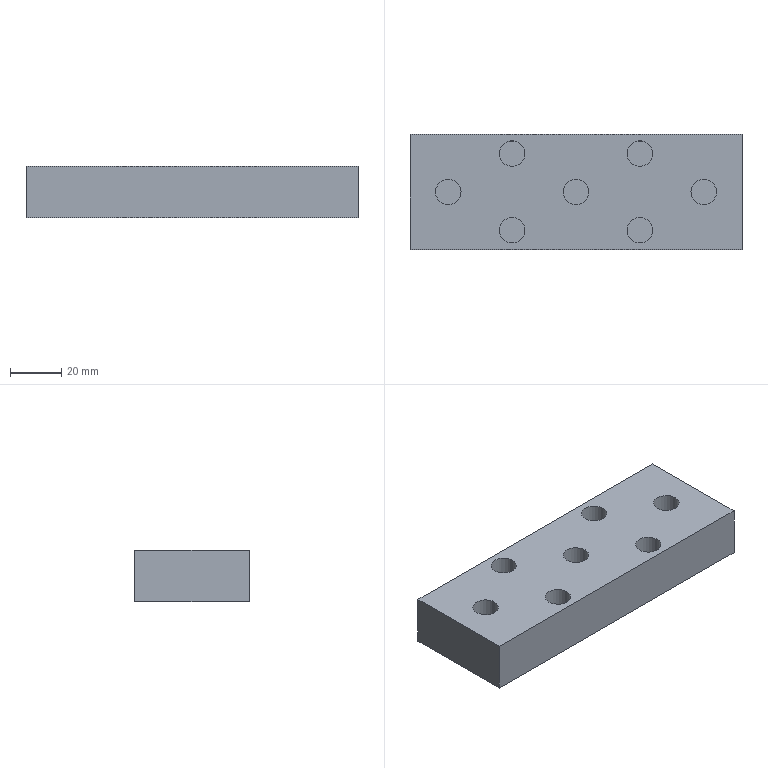Part | NX | 1 solid | 20 faces | box 130 x 45 x 20 mm | volume 111502 mm3 | plane 13 | cylinder 7 | commonest cylinder face diameters 10 x7
STEP:
#1=CARTESIAN_POINT('',(95.,37.5,20.));
#2=VERTEX_POINT('',#1);
#3=CARTESIAN_POINT('',(90.,37.5,20.));
#4=DIRECTION('',(0.,0.,-1.));
#5=DIRECTION('',(1.,0.,0.));
#6=AXIS2_PLACEMENT_3D('',#3,#4,#5);
#7=CIRCLE('',#6,5.);
#8=EDGE_CURVE('',#2,#2,#7,.T.);
#9=ORIENTED_EDGE('',*,*,#8,.T.);
#10=EDGE_LOOP('',(#9));
#11=FACE_BOUND('',#10,.T.);
#12=CARTESIAN_POINT('',(45.,37.5,20.));
#13=VERTEX_POINT('',#12);
#14=CARTESIAN_POINT('',(40.,37.5,20.));
#15=DIRECTION('',(0.,0.,-1.));
#16=DIRECTION('',(1.,0.,0.));
#17=AXIS2_PLACEMENT_3D('',#14,#15,#16);
#18=CIRCLE('',#17,5.);
#19=EDGE_CURVE('',#13,#13,#18,.T.);
#20=ORIENTED_EDGE('',*,*,#19,.T.);
#21=EDGE_LOOP('',(#20));
#22=FACE_BOUND('',#21,.T.);
#23=CARTESIAN_POINT('',(95.,7.5,20.));
#24=VERTEX_POINT('',#23);
#25=CARTESIAN_POINT('',(90.,7.5,20.));
#26=DIRECTION('',(0.,0.,-1.));
#27=DIRECTION('',(1.,0.,0.));
#28=AXIS2_PLACEMENT_3D('',#25,#26,#27);
#29=CIRCLE('',#28,5.);
#30=EDGE_CURVE('',#24,#24,#29,.T.);
#31=ORIENTED_EDGE('',*,*,#30,.T.);
#32=EDGE_LOOP('',(#31));
#33=FACE_BOUND('',#32,.T.);
#34=CARTESIAN_POINT('',(45.,7.5,20.));
#35=VERTEX_POINT('',#34);
#36=CARTESIAN_POINT('',(40.,7.5,20.));
#37=DIRECTION('',(0.,0.,-1.));
#38=DIRECTION('',(1.,0.,0.));
#39=AXIS2_PLACEMENT_3D('',#36,#37,#38);
#40=CIRCLE('',#39,5.);
#41=EDGE_CURVE('',#35,#35,#40,.T.);
#42=ORIENTED_EDGE('',*,*,#41,.T.);
#43=EDGE_LOOP('',(#42));
#44=FACE_BOUND('',#43,.T.);
#45=CARTESIAN_POINT('',(120.,22.5,20.));
#46=VERTEX_POINT('',#45);
#47=CARTESIAN_POINT('',(115.,22.5,20.));
#48=DIRECTION('',(0.,0.,-1.));
#49=DIRECTION('',(1.,0.,0.));
#50=AXIS2_PLACEMENT_3D('',#47,#48,#49);
#51=CIRCLE('',#50,5.);
#52=EDGE_CURVE('',#46,#46,#51,.T.);
#53=ORIENTED_EDGE('',*,*,#52,.T.);
#54=EDGE_LOOP('',(#53));
#55=FACE_BOUND('',#54,.T.);
#56=CARTESIAN_POINT('',(20.,22.5,20.));
#57=VERTEX_POINT('',#56);
#58=CARTESIAN_POINT('',(15.,22.5,20.));
#59=DIRECTION('',(0.,0.,-1.));
#60=DIRECTION('',(1.,0.,0.));
#61=AXIS2_PLACEMENT_3D('',#58,#59,#60);
#62=CIRCLE('',#61,5.);
#63=EDGE_CURVE('',#57,#57,#62,.T.);
#64=ORIENTED_EDGE('',*,*,#63,.T.);
#65=EDGE_LOOP('',(#64));
#66=FACE_BOUND('',#65,.T.);
#67=CARTESIAN_POINT('',(70.,22.5,20.));
#68=VERTEX_POINT('',#67);
#69=CARTESIAN_POINT('',(65.,22.5,20.));
#70=DIRECTION('',(0.,0.,-1.));
#71=DIRECTION('',(1.,0.,0.));
#72=AXIS2_PLACEMENT_3D('',#69,#70,#71);
#73=CIRCLE('',#72,5.);
#74=EDGE_CURVE('',#68,#68,#73,.T.);
#75=ORIENTED_EDGE('',*,*,#74,.T.);
#76=EDGE_LOOP('',(#75));
#77=FACE_BOUND('',#76,.T.);
#78=CARTESIAN_POINT('',(130.,0.,20.));
#79=VERTEX_POINT('',#78);
#80=CARTESIAN_POINT('',(0.,0.,20.));
#81=VERTEX_POINT('',#80);
#82=CARTESIAN_POINT('',(65.,0.,20.));
#83=DIRECTION('',(-1.,0.,0.));
#84=VECTOR('',#83,1000.);
#85=LINE('',#82,#84);
#86=EDGE_CURVE('',#79,#81,#85,.T.);
#87=ORIENTED_EDGE('',*,*,#86,.F.);
#88=CARTESIAN_POINT('',(130.,45.,20.));
#89=VERTEX_POINT('',#88);
#90=CARTESIAN_POINT('',(130.,22.5,20.));
#91=DIRECTION('',(0.,-1.,0.));
#92=VECTOR('',#91,1000.);
#93=LINE('',#90,#92);
#94=EDGE_CURVE('',#89,#79,#93,.T.);
#95=ORIENTED_EDGE('',*,*,#94,.F.);
#96=CARTESIAN_POINT('',(0.,45.,20.));
#97=VERTEX_POINT('',#96);
#98=CARTESIAN_POINT('',(65.,45.,20.));
#99=DIRECTION('',(1.,0.,0.));
#100=VECTOR('',#99,1000.);
#101=LINE('',#98,#100);
#102=EDGE_CURVE('',#97,#89,#101,.T.);
#103=ORIENTED_EDGE('',*,*,#102,.F.);
#104=CARTESIAN_POINT('',(0.,22.5,20.));
#105=DIRECTION('',(0.,1.,0.));
#106=VECTOR('',#105,1000.);
#107=LINE('',#104,#106);
#108=EDGE_CURVE('',#81,#97,#107,.T.);
#109=ORIENTED_EDGE('',*,*,#108,.F.);
#110=EDGE_LOOP('',(#87,#95,#103,#109));
#111=FACE_BOUND('',#110,.T.);
#112=CARTESIAN_POINT('',(65.,22.5,20.));
#113=DIRECTION('',(0.,0.,1.));
#114=DIRECTION('',(1.,0.,0.));
#115=AXIS2_PLACEMENT_3D('',#112,#113,#114);
#116=PLANE('',#115);
#117=ADVANCED_FACE('',(#11,#22,#33,#44,#55,#66,#77,#111),#116,.T.);
#118=CARTESIAN_POINT('',(130.,0.,0.));
#119=VERTEX_POINT('',#118);
#120=CARTESIAN_POINT('',(130.,0.,0.));
#121=DIRECTION('',(0.,0.,1.));
#122=VECTOR('',#121,1000.);
#123=LINE('',#120,#122);
#124=EDGE_CURVE('',#119,#79,#123,.T.);
#125=ORIENTED_EDGE('',*,*,#124,.T.);
#126=ORIENTED_EDGE('',*,*,#86,.T.);
#127=CARTESIAN_POINT('',(0.,0.,0.));
#128=VERTEX_POINT('',#127);
#129=CARTESIAN_POINT('',(0.,0.,0.));
#130=DIRECTION('',(0.,0.,1.));
#131=VECTOR('',#130,1000.);
#132=LINE('',#129,#131);
#133=EDGE_CURVE('',#128,#81,#132,.T.);
#134=ORIENTED_EDGE('',*,*,#133,.F.);
#135=CARTESIAN_POINT('',(65.,0.,0.));
#136=DIRECTION('',(1.,0.,0.));
#137=VECTOR('',#136,1000.);
#138=LINE('',#135,#137);
#139=EDGE_CURVE('',#128,#119,#138,.T.);
#140=ORIENTED_EDGE('',*,*,#139,.T.);
#141=EDGE_LOOP('',(#125,#126,#134,#140));
#142=FACE_BOUND('',#141,.T.);
#143=CARTESIAN_POINT('',(65.,0.,0.));
#144=DIRECTION('',(0.,-1.,0.));
#145=DIRECTION('',(0.,0.,-1.));
#146=AXIS2_PLACEMENT_3D('',#143,#144,#145);
#147=PLANE('',#146);
#148=ADVANCED_FACE('',(#142),#147,.T.);
#149=ORIENTED_EDGE('',*,*,#133,.T.);
#150=ORIENTED_EDGE('',*,*,#108,.T.);
#151=CARTESIAN_POINT('',(0.,45.,0.));
#152=VERTEX_POINT('',#151);
#153=CARTESIAN_POINT('',(0.,45.,0.));
#154=DIRECTION('',(0.,0.,1.));
#155=VECTOR('',#154,1000.);
#156=LINE('',#153,#155);
#157=EDGE_CURVE('',#152,#97,#156,.T.);
#158=ORIENTED_EDGE('',*,*,#157,.F.);
#159=CARTESIAN_POINT('',(0.,22.5,0.));
#160=DIRECTION('',(0.,-1.,0.));
#161=VECTOR('',#160,1000.);
#162=LINE('',#159,#161);
#163=EDGE_CURVE('',#152,#128,#162,.T.);
#164=ORIENTED_EDGE('',*,*,#163,.T.);
#165=EDGE_LOOP('',(#149,#150,#158,#164));
#166=FACE_BOUND('',#165,.T.);
#167=CARTESIAN_POINT('',(0.,22.5,0.));
#168=DIRECTION('',(-1.,0.,0.));
#169=DIRECTION('',(0.,0.,1.));
#170=AXIS2_PLACEMENT_3D('',#167,#168,#169);
#171=PLANE('',#170);
#172=ADVANCED_FACE('',(#166),#171,.T.);
#173=ORIENTED_EDGE('',*,*,#157,.T.);
#174=ORIENTED_EDGE('',*,*,#102,.T.);
#175=CARTESIAN_POINT('',(130.,45.,0.));
#176=VERTEX_POINT('',#175);
#177=CARTESIAN_POINT('',(130.,45.,0.));
#178=DIRECTION('',(0.,0.,1.));
#179=VECTOR('',#178,1000.);
#180=LINE('',#177,#179);
#181=EDGE_CURVE('',#176,#89,#180,.T.);
#182=ORIENTED_EDGE('',*,*,#181,.F.);
#183=CARTESIAN_POINT('',(65.,45.,0.));
#184=DIRECTION('',(-1.,0.,0.));
#185=VECTOR('',#184,1000.);
#186=LINE('',#183,#185);
#187=EDGE_CURVE('',#176,#152,#186,.T.);
#188=ORIENTED_EDGE('',*,*,#187,.T.);
#189=EDGE_LOOP('',(#173,#174,#182,#188));
#190=FACE_BOUND('',#189,.T.);
#191=CARTESIAN_POINT('',(65.,45.,0.));
#192=DIRECTION('',(0.,1.,0.));
#193=DIRECTION('',(0.,0.,1.));
#194=AXIS2_PLACEMENT_3D('',#191,#192,#193);
#195=PLANE('',#194);
#196=ADVANCED_FACE('',(#190),#195,.T.);
#197=CARTESIAN_POINT('',(130.,22.5,0.));
#198=DIRECTION('',(0.,1.,0.));
#199=VECTOR('',#198,1000.);
#200=LINE('',#197,#199);
#201=EDGE_CURVE('',#119,#176,#200,.T.);
#202=ORIENTED_EDGE('',*,*,#201,.F.);
#203=ORIENTED_EDGE('',*,*,#139,.F.);
#204=ORIENTED_EDGE('',*,*,#163,.F.);
#205=ORIENTED_EDGE('',*,*,#187,.F.);
#206=EDGE_LOOP('',(#202,#203,#204,#205));
#207=FACE_BOUND('',#206,.T.);
#208=CARTESIAN_POINT('',(65.,22.5,0.));
#209=DIRECTION('',(0.,0.,-1.));
#210=DIRECTION('',(-1.,0.,0.));
#211=AXIS2_PLACEMENT_3D('',#208,#209,#210);
#212=PLANE('',#211);
#213=ADVANCED_FACE('',(#207),#212,.T.);
#214=ORIENTED_EDGE('',*,*,#201,.T.);
#215=ORIENTED_EDGE('',*,*,#181,.T.);
#216=ORIENTED_EDGE('',*,*,#94,.T.);
#217=ORIENTED_EDGE('',*,*,#124,.F.);
#218=EDGE_LOOP('',(#214,#215,#216,#217));
#219=FACE_BOUND('',#218,.T.);
#220=CARTESIAN_POINT('',(130.,22.5,0.));
#221=DIRECTION('',(1.,0.,0.));
#222=DIRECTION('',(0.,0.,-1.));
#223=AXIS2_PLACEMENT_3D('',#220,#221,#222);
#224=PLANE('',#223);
#225=ADVANCED_FACE('',(#219),#224,.T.);
#226=CARTESIAN_POINT('',(70.,22.5,10.));
#227=VERTEX_POINT('',#226);
#228=CARTESIAN_POINT('',(65.,22.5,10.));
#229=DIRECTION('',(0.,0.,1.));
#230=DIRECTION('',(1.,0.,0.));
#231=AXIS2_PLACEMENT_3D('',#228,#229,#230);
#232=CIRCLE('',#231,5.);
#233=EDGE_CURVE('',#227,#227,#232,.F.);
#234=ORIENTED_EDGE('',*,*,#233,.F.);
#235=EDGE_LOOP('',(#234));
#236=FACE_BOUND('',#235,.T.);
#237=CARTESIAN_POINT('',(65.,22.5,10.));
#238=DIRECTION('',(0.,0.,-1.));
#239=DIRECTION('',(-1.,0.,0.));
#240=AXIS2_PLACEMENT_3D('',#237,#238,#239);
#241=PLANE('',#240);
#242=ADVANCED_FACE('',(#236),#241,.F.);
#243=ORIENTED_EDGE('',*,*,#233,.T.);
#244=EDGE_LOOP('',(#243));
#245=FACE_BOUND('',#244,.T.);
#246=ORIENTED_EDGE('',*,*,#74,.F.);
#247=EDGE_LOOP('',(#246));
#248=FACE_BOUND('',#247,.T.);
#249=CARTESIAN_POINT('',(65.,22.5,20.));
#250=DIRECTION('',(0.,0.,-1.));
#251=DIRECTION('',(1.,0.,0.));
#252=AXIS2_PLACEMENT_3D('',#249,#250,#251);
#253=CYLINDRICAL_SURFACE('',#252,5.);
#254=ADVANCED_FACE('',(#245,#248),#253,.F.);
#255=CARTESIAN_POINT('',(20.,22.5,10.));
#256=VERTEX_POINT('',#255);
#257=CARTESIAN_POINT('',(15.,22.5,10.));
#258=DIRECTION('',(0.,0.,1.));
#259=DIRECTION('',(1.,0.,0.));
#260=AXIS2_PLACEMENT_3D('',#257,#258,#259);
#261=CIRCLE('',#260,5.);
#262=EDGE_CURVE('',#256,#256,#261,.F.);
#263=ORIENTED_EDGE('',*,*,#262,.F.);
#264=EDGE_LOOP('',(#263));
#265=FACE_BOUND('',#264,.T.);
#266=CARTESIAN_POINT('',(15.,22.5,10.));
#267=DIRECTION('',(0.,0.,-1.));
#268=DIRECTION('',(-1.,0.,0.));
#269=AXIS2_PLACEMENT_3D('',#266,#267,#268);
#270=PLANE('',#269);
#271=ADVANCED_FACE('',(#265),#270,.F.);
#272=ORIENTED_EDGE('',*,*,#262,.T.);
#273=EDGE_LOOP('',(#272));
#274=FACE_BOUND('',#273,.T.);
#275=ORIENTED_EDGE('',*,*,#63,.F.);
#276=EDGE_LOOP('',(#275));
#277=FACE_BOUND('',#276,.T.);
#278=CARTESIAN_POINT('',(15.,22.5,20.));
#279=DIRECTION('',(0.,0.,-1.));
#280=DIRECTION('',(1.,0.,0.));
#281=AXIS2_PLACEMENT_3D('',#278,#279,#280);
#282=CYLINDRICAL_SURFACE('',#281,5.);
#283=ADVANCED_FACE('',(#274,#277),#282,.F.);
#284=CARTESIAN_POINT('',(120.,22.5,10.));
#285=VERTEX_POINT('',#284);
#286=CARTESIAN_POINT('',(115.,22.5,10.));
#287=DIRECTION('',(0.,0.,1.));
#288=DIRECTION('',(1.,0.,0.));
#289=AXIS2_PLACEMENT_3D('',#286,#287,#288);
#290=CIRCLE('',#289,5.);
#291=EDGE_CURVE('',#285,#285,#290,.F.);
#292=ORIENTED_EDGE('',*,*,#291,.F.);
#293=EDGE_LOOP('',(#292));
#294=FACE_BOUND('',#293,.T.);
#295=CARTESIAN_POINT('',(115.,22.5,10.));
#296=DIRECTION('',(0.,0.,-1.));
#297=DIRECTION('',(-1.,0.,0.));
#298=AXIS2_PLACEMENT_3D('',#295,#296,#297);
#299=PLANE('',#298);
#300=ADVANCED_FACE('',(#294),#299,.F.);
#301=ORIENTED_EDGE('',*,*,#291,.T.);
#302=EDGE_LOOP('',(#301));
#303=FACE_BOUND('',#302,.T.);
#304=ORIENTED_EDGE('',*,*,#52,.F.);
#305=EDGE_LOOP('',(#304));
#306=FACE_BOUND('',#305,.T.);
#307=CARTESIAN_POINT('',(115.,22.5,20.));
#308=DIRECTION('',(0.,0.,-1.));
#309=DIRECTION('',(1.,0.,0.));
#310=AXIS2_PLACEMENT_3D('',#307,#308,#309);
#311=CYLINDRICAL_SURFACE('',#310,5.);
#312=ADVANCED_FACE('',(#303,#306),#311,.F.);
#313=CARTESIAN_POINT('',(45.,7.5,10.));
#314=VERTEX_POINT('',#313);
#315=CARTESIAN_POINT('',(40.,7.5,10.));
#316=DIRECTION('',(0.,0.,1.));
#317=DIRECTION('',(1.,0.,0.));
#318=AXIS2_PLACEMENT_3D('',#315,#316,#317);
#319=CIRCLE('',#318,5.);
#320=EDGE_CURVE('',#314,#314,#319,.F.);
#321=ORIENTED_EDGE('',*,*,#320,.F.);
#322=EDGE_LOOP('',(#321));
#323=FACE_BOUND('',#322,.T.);
#324=CARTESIAN_POINT('',(40.,7.5,10.));
#325=DIRECTION('',(0.,0.,-1.));
#326=DIRECTION('',(-1.,0.,0.));
#327=AXIS2_PLACEMENT_3D('',#324,#325,#326);
#328=PLANE('',#327);
#329=ADVANCED_FACE('',(#323),#328,.F.);
#330=ORIENTED_EDGE('',*,*,#320,.T.);
#331=EDGE_LOOP('',(#330));
#332=FACE_BOUND('',#331,.T.);
#333=ORIENTED_EDGE('',*,*,#41,.F.);
#334=EDGE_LOOP('',(#333));
#335=FACE_BOUND('',#334,.T.);
#336=CARTESIAN_POINT('',(40.,7.5,20.));
#337=DIRECTION('',(0.,0.,-1.));
#338=DIRECTION('',(1.,0.,0.));
#339=AXIS2_PLACEMENT_3D('',#336,#337,#338);
#340=CYLINDRICAL_SURFACE('',#339,5.);
#341=ADVANCED_FACE('',(#332,#335),#340,.F.);
#342=CARTESIAN_POINT('',(95.,7.5,10.));
#343=VERTEX_POINT('',#342);
#344=CARTESIAN_POINT('',(90.,7.5,10.));
#345=DIRECTION('',(0.,0.,1.));
#346=DIRECTION('',(1.,0.,0.));
#347=AXIS2_PLACEMENT_3D('',#344,#345,#346);
#348=CIRCLE('',#347,5.);
#349=EDGE_CURVE('',#343,#343,#348,.F.);
#350=ORIENTED_EDGE('',*,*,#349,.F.);
#351=EDGE_LOOP('',(#350));
#352=FACE_BOUND('',#351,.T.);
#353=CARTESIAN_POINT('',(90.,7.5,10.));
#354=DIRECTION('',(0.,0.,-1.));
#355=DIRECTION('',(-1.,0.,0.));
#356=AXIS2_PLACEMENT_3D('',#353,#354,#355);
#357=PLANE('',#356);
#358=ADVANCED_FACE('',(#352),#357,.F.);
#359=ORIENTED_EDGE('',*,*,#349,.T.);
#360=EDGE_LOOP('',(#359));
#361=FACE_BOUND('',#360,.T.);
#362=ORIENTED_EDGE('',*,*,#30,.F.);
#363=EDGE_LOOP('',(#362));
#364=FACE_BOUND('',#363,.T.);
#365=CARTESIAN_POINT('',(90.,7.5,20.));
#366=DIRECTION('',(0.,0.,-1.));
#367=DIRECTION('',(1.,0.,0.));
#368=AXIS2_PLACEMENT_3D('',#365,#366,#367);
#369=CYLINDRICAL_SURFACE('',#368,5.);
#370=ADVANCED_FACE('',(#361,#364),#369,.F.);
#371=CARTESIAN_POINT('',(45.,37.5,10.));
#372=VERTEX_POINT('',#371);
#373=CARTESIAN_POINT('',(40.,37.5,10.));
#374=DIRECTION('',(0.,0.,1.));
#375=DIRECTION('',(1.,0.,0.));
#376=AXIS2_PLACEMENT_3D('',#373,#374,#375);
#377=CIRCLE('',#376,5.);
#378=EDGE_CURVE('',#372,#372,#377,.F.);
#379=ORIENTED_EDGE('',*,*,#378,.F.);
#380=EDGE_LOOP('',(#379));
#381=FACE_BOUND('',#380,.T.);
#382=CARTESIAN_POINT('',(40.,37.5,10.));
#383=DIRECTION('',(0.,0.,-1.));
#384=DIRECTION('',(-1.,0.,0.));
#385=AXIS2_PLACEMENT_3D('',#382,#383,#384);
#386=PLANE('',#385);
#387=ADVANCED_FACE('',(#381),#386,.F.);
#388=ORIENTED_EDGE('',*,*,#378,.T.);
#389=EDGE_LOOP('',(#388));
#390=FACE_BOUND('',#389,.T.);
#391=ORIENTED_EDGE('',*,*,#19,.F.);
#392=EDGE_LOOP('',(#391));
#393=FACE_BOUND('',#392,.T.);
#394=CARTESIAN_POINT('',(40.,37.5,20.));
#395=DIRECTION('',(0.,0.,-1.));
#396=DIRECTION('',(1.,0.,0.));
#397=AXIS2_PLACEMENT_3D('',#394,#395,#396);
#398=CYLINDRICAL_SURFACE('',#397,5.);
#399=ADVANCED_FACE('',(#390,#393),#398,.F.);
#400=CARTESIAN_POINT('',(95.,37.5,10.));
#401=VERTEX_POINT('',#400);
#402=CARTESIAN_POINT('',(90.,37.5,10.));
#403=DIRECTION('',(0.,0.,1.));
#404=DIRECTION('',(1.,0.,0.));
#405=AXIS2_PLACEMENT_3D('',#402,#403,#404);
#406=CIRCLE('',#405,5.);
#407=EDGE_CURVE('',#401,#401,#406,.F.);
#408=ORIENTED_EDGE('',*,*,#407,.F.);
#409=EDGE_LOOP('',(#408));
#410=FACE_BOUND('',#409,.T.);
#411=CARTESIAN_POINT('',(90.,37.5,10.));
#412=DIRECTION('',(0.,0.,-1.));
#413=DIRECTION('',(-1.,0.,0.));
#414=AXIS2_PLACEMENT_3D('',#411,#412,#413);
#415=PLANE('',#414);
#416=ADVANCED_FACE('',(#410),#415,.F.);
#417=ORIENTED_EDGE('',*,*,#407,.T.);
#418=EDGE_LOOP('',(#417));
#419=FACE_BOUND('',#418,.T.);
#420=ORIENTED_EDGE('',*,*,#8,.F.);
#421=EDGE_LOOP('',(#420));
#422=FACE_BOUND('',#421,.T.);
#423=CARTESIAN_POINT('',(90.,37.5,20.));
#424=DIRECTION('',(0.,0.,-1.));
#425=DIRECTION('',(1.,0.,0.));
#426=AXIS2_PLACEMENT_3D('',#423,#424,#425);
#427=CYLINDRICAL_SURFACE('',#426,5.);
#428=ADVANCED_FACE('',(#419,#422),#427,.F.);
#429=CLOSED_SHELL('',(#117,#148,#172,#196,#213,#225,#242,#254,#271,#283,#300,#312,#329,#341,#358,#370,#387,#399,#416,#428));
#430=MANIFOLD_SOLID_BREP('',#429);
#431=(LENGTH_UNIT()NAMED_UNIT(*)SI_UNIT(.MILLI.,.METRE.));
#432=UNCERTAINTY_MEASURE_WITH_UNIT(LENGTH_MEASURE(0.00001),#431,'','');
#433=(NAMED_UNIT(*)PLANE_ANGLE_UNIT()SI_UNIT($,.RADIAN.));
#434=(NAMED_UNIT(*)SI_UNIT($,.STERADIAN.)SOLID_ANGLE_UNIT());
#435=(GEOMETRIC_REPRESENTATION_CONTEXT(3)GLOBAL_UNCERTAINTY_ASSIGNED_CONTEXT((#432))GLOBAL_UNIT_ASSIGNED_CONTEXT((#431,#433,#434))REPRESENTATION_CONTEXT('',''));
#436=ADVANCED_BREP_SHAPE_REPRESENTATION('',(#430),#435);